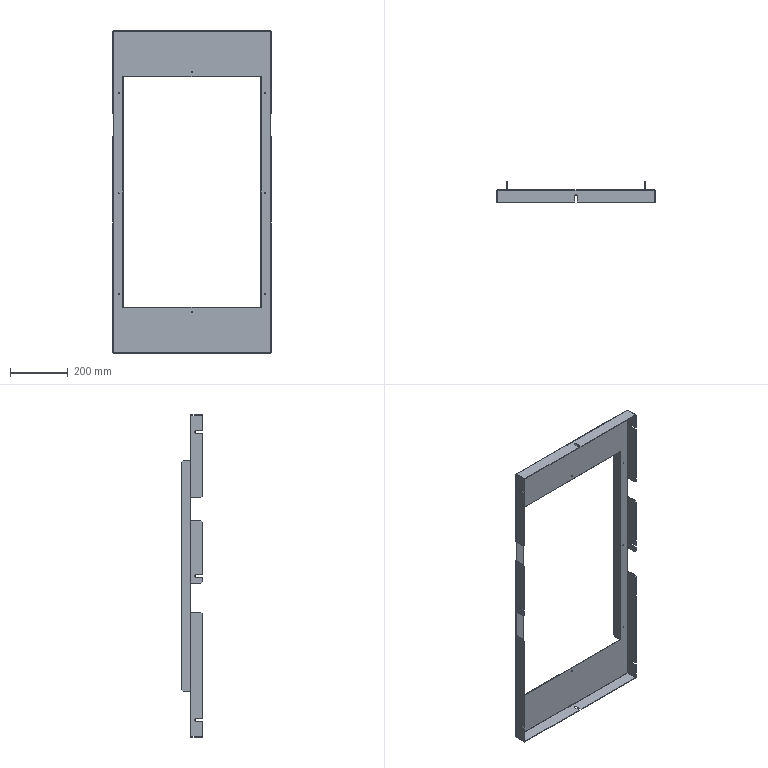Part | NX | 1 solid | 142 faces | box 549 x 72 x 1119 mm | volume 790596 mm3 | plane 102 | cylinder 32 | spline 8 | commonest cylinder face diameters 0.4 x8 3.3 x8 4.4 x8 8.5 x8